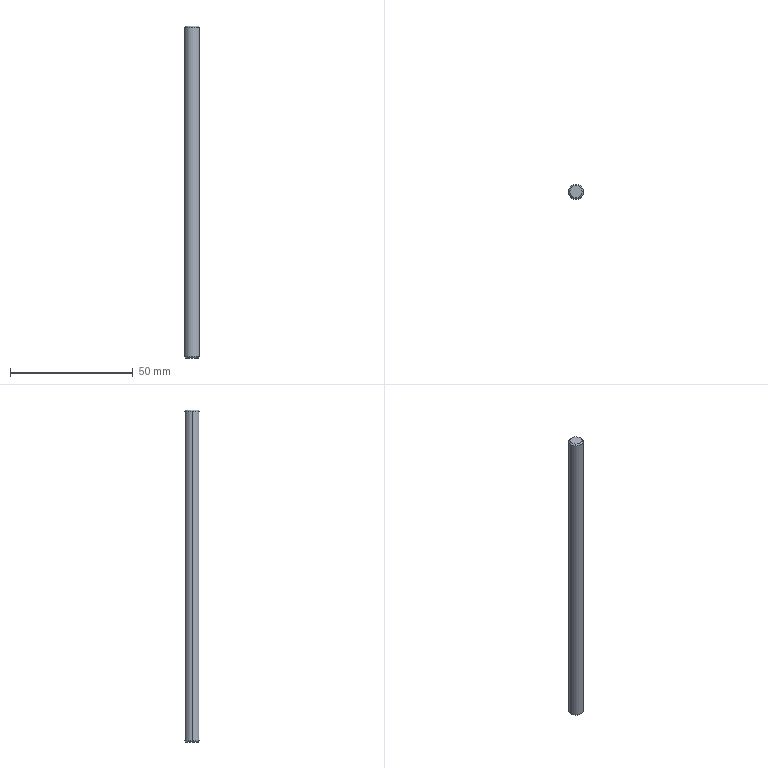Part | 1 solid | 8 faces | box 6 x 6 x 135 mm | volume 3813 mm3 | cone 4 | cylinder 2 | plane 2 | commonest cylinder face diameters 6 x2
STEP:
#1=CARTESIAN_POINT('',(2.5,0.,67.5));
#2=VERTEX_POINT('',#1);
#3=CARTESIAN_POINT('',(-2.5,0.,67.5));
#4=VERTEX_POINT('',#3);
#5=CARTESIAN_POINT('',(0.,0.,67.5));
#6=DIRECTION('',(0.,0.,1.));
#7=DIRECTION('',(1.,0.,0.));
#8=AXIS2_PLACEMENT_3D('',#5,#6,#7);
#9=CIRCLE('',#8,2.5);
#10=EDGE_CURVE('',#2,#4,#9,.T.);
#11=ORIENTED_EDGE('',*,*,#10,.F.);
#12=CARTESIAN_POINT('',(3.,0.,67.));
#13=VERTEX_POINT('',#12);
#14=CARTESIAN_POINT('',(2.5,0.,67.5));
#15=DIRECTION('',(0.7071,0.,-0.7071));
#16=VECTOR('',#15,1000.);
#17=LINE('',#14,#16);
#18=EDGE_CURVE('',#2,#13,#17,.T.);
#19=ORIENTED_EDGE('',*,*,#18,.T.);
#20=CARTESIAN_POINT('',(-3.,0.,67.));
#21=VERTEX_POINT('',#20);
#22=CARTESIAN_POINT('',(0.,0.,67.));
#23=DIRECTION('',(0.,0.,-1.));
#24=DIRECTION('',(1.,0.,0.));
#25=AXIS2_PLACEMENT_3D('',#22,#23,#24);
#26=CIRCLE('',#25,3.);
#27=EDGE_CURVE('',#21,#13,#26,.T.);
#28=ORIENTED_EDGE('',*,*,#27,.F.);
#29=CARTESIAN_POINT('',(-2.5,0.,67.5));
#30=DIRECTION('',(-0.7071,0.,-0.7071));
#31=VECTOR('',#30,1000.);
#32=LINE('',#29,#31);
#33=EDGE_CURVE('',#4,#21,#32,.T.);
#34=ORIENTED_EDGE('',*,*,#33,.F.);
#35=EDGE_LOOP('',(#11,#19,#28,#34));
#36=FACE_OUTER_BOUND('',#35,.T.);
#37=CARTESIAN_POINT('',(0.,0.,67.5));
#38=DIRECTION('',(0.,0.,-1.));
#39=DIRECTION('',(-1.,0.,0.));
#40=AXIS2_PLACEMENT_3D('',#37,#38,#39);
#41=CONICAL_SURFACE('',#40,2.5,0.7854);
#42=ADVANCED_FACE('',(#36),#41,.T.);
#43=CARTESIAN_POINT('',(-2.5,0.,-67.5));
#44=VERTEX_POINT('',#43);
#45=CARTESIAN_POINT('',(2.5,0.,-67.5));
#46=VERTEX_POINT('',#45);
#47=CARTESIAN_POINT('',(0.,0.,-67.5));
#48=DIRECTION('',(0.,0.,-1.));
#49=DIRECTION('',(1.,0.,0.));
#50=AXIS2_PLACEMENT_3D('',#47,#48,#49);
#51=CIRCLE('',#50,2.5);
#52=EDGE_CURVE('',#44,#46,#51,.T.);
#53=ORIENTED_EDGE('',*,*,#52,.F.);
#54=CARTESIAN_POINT('',(-3.,0.,-67.));
#55=VERTEX_POINT('',#54);
#56=CARTESIAN_POINT('',(-3.,0.,-67.));
#57=DIRECTION('',(-0.7071,0.,0.7071));
#58=VECTOR('',#57,1000.);
#59=LINE('',#56,#58);
#60=EDGE_CURVE('',#44,#55,#59,.T.);
#61=ORIENTED_EDGE('',*,*,#60,.T.);
#62=CARTESIAN_POINT('',(3.,0.,-67.));
#63=VERTEX_POINT('',#62);
#64=CARTESIAN_POINT('',(0.,0.,-67.));
#65=DIRECTION('',(0.,0.,1.));
#66=DIRECTION('',(1.,0.,0.));
#67=AXIS2_PLACEMENT_3D('',#64,#65,#66);
#68=CIRCLE('',#67,3.);
#69=EDGE_CURVE('',#63,#55,#68,.T.);
#70=ORIENTED_EDGE('',*,*,#69,.F.);
#71=CARTESIAN_POINT('',(3.,0.,-67.));
#72=DIRECTION('',(0.7071,0.,0.7071));
#73=VECTOR('',#72,1000.);
#74=LINE('',#71,#73);
#75=EDGE_CURVE('',#46,#63,#74,.T.);
#76=ORIENTED_EDGE('',*,*,#75,.F.);
#77=EDGE_LOOP('',(#53,#61,#70,#76));
#78=FACE_OUTER_BOUND('',#77,.T.);
#79=CARTESIAN_POINT('',(0.,0.,-67.));
#80=DIRECTION('',(0.,0.,1.));
#81=DIRECTION('',(1.,0.,0.));
#82=AXIS2_PLACEMENT_3D('',#79,#80,#81);
#83=CONICAL_SURFACE('',#82,3.,0.7854);
#84=ADVANCED_FACE('',(#78),#83,.T.);
#85=ORIENTED_EDGE('',*,*,#27,.T.);
#86=CARTESIAN_POINT('',(3.,0.,67.5));
#87=DIRECTION('',(0.,0.,-1.));
#88=VECTOR('',#87,1000.);
#89=LINE('',#86,#88);
#90=EDGE_CURVE('',#13,#63,#89,.T.);
#91=ORIENTED_EDGE('',*,*,#90,.T.);
#92=ORIENTED_EDGE('',*,*,#69,.T.);
#93=CARTESIAN_POINT('',(-3.,0.,67.5));
#94=DIRECTION('',(0.,0.,-1.));
#95=VECTOR('',#94,1000.);
#96=LINE('',#93,#95);
#97=EDGE_CURVE('',#21,#55,#96,.T.);
#98=ORIENTED_EDGE('',*,*,#97,.F.);
#99=EDGE_LOOP('',(#85,#91,#92,#98));
#100=FACE_OUTER_BOUND('',#99,.T.);
#101=CARTESIAN_POINT('',(0.,0.,67.5));
#102=DIRECTION('',(0.,0.,-1.));
#103=DIRECTION('',(-1.,0.,0.));
#104=AXIS2_PLACEMENT_3D('',#101,#102,#103);
#105=CYLINDRICAL_SURFACE('',#104,3.);
#106=ADVANCED_FACE('',(#100),#105,.T.);
#107=ORIENTED_EDGE('',*,*,#90,.F.);
#108=CARTESIAN_POINT('',(0.,0.,67.));
#109=DIRECTION('',(0.,0.,-1.));
#110=DIRECTION('',(1.,0.,0.));
#111=AXIS2_PLACEMENT_3D('',#108,#109,#110);
#112=CIRCLE('',#111,3.);
#113=EDGE_CURVE('',#13,#21,#112,.T.);
#114=ORIENTED_EDGE('',*,*,#113,.T.);
#115=ORIENTED_EDGE('',*,*,#97,.T.);
#116=CARTESIAN_POINT('',(0.,0.,-67.));
#117=DIRECTION('',(0.,0.,1.));
#118=DIRECTION('',(1.,0.,0.));
#119=AXIS2_PLACEMENT_3D('',#116,#117,#118);
#120=CIRCLE('',#119,3.);
#121=EDGE_CURVE('',#55,#63,#120,.T.);
#122=ORIENTED_EDGE('',*,*,#121,.T.);
#123=EDGE_LOOP('',(#107,#114,#115,#122));
#124=FACE_OUTER_BOUND('',#123,.T.);
#125=CARTESIAN_POINT('',(0.,0.,67.5));
#126=DIRECTION('',(0.,0.,-1.));
#127=DIRECTION('',(-1.,0.,0.));
#128=AXIS2_PLACEMENT_3D('',#125,#126,#127);
#129=CYLINDRICAL_SURFACE('',#128,3.);
#130=ADVANCED_FACE('',(#124),#129,.T.);
#131=CARTESIAN_POINT('',(0.,0.,67.5));
#132=DIRECTION('',(0.,0.,1.));
#133=DIRECTION('',(1.,0.,0.));
#134=AXIS2_PLACEMENT_3D('',#131,#132,#133);
#135=CIRCLE('',#134,2.5);
#136=EDGE_CURVE('',#4,#2,#135,.T.);
#137=ORIENTED_EDGE('',*,*,#136,.T.);
#138=ORIENTED_EDGE('',*,*,#10,.T.);
#139=EDGE_LOOP('',(#137,#138));
#140=FACE_OUTER_BOUND('',#139,.T.);
#141=CARTESIAN_POINT('',(0.,0.,67.5));
#142=DIRECTION('',(0.,0.,1.));
#143=DIRECTION('',(1.,0.,0.));
#144=AXIS2_PLACEMENT_3D('',#141,#142,#143);
#145=PLANE('',#144);
#146=ADVANCED_FACE('',(#140),#145,.T.);
#147=CARTESIAN_POINT('',(0.,0.,-67.5));
#148=DIRECTION('',(0.,0.,-1.));
#149=DIRECTION('',(1.,0.,0.));
#150=AXIS2_PLACEMENT_3D('',#147,#148,#149);
#151=CIRCLE('',#150,2.5);
#152=EDGE_CURVE('',#46,#44,#151,.T.);
#153=ORIENTED_EDGE('',*,*,#152,.T.);
#154=ORIENTED_EDGE('',*,*,#52,.T.);
#155=EDGE_LOOP('',(#153,#154));
#156=FACE_OUTER_BOUND('',#155,.T.);
#157=CARTESIAN_POINT('',(0.,0.,-67.5));
#158=DIRECTION('',(0.,0.,1.));
#159=DIRECTION('',(1.,0.,0.));
#160=AXIS2_PLACEMENT_3D('',#157,#158,#159);
#161=PLANE('',#160);
#162=ADVANCED_FACE('',(#156),#161,.F.);
#163=ORIENTED_EDGE('',*,*,#60,.F.);
#164=ORIENTED_EDGE('',*,*,#152,.F.);
#165=ORIENTED_EDGE('',*,*,#75,.T.);
#166=ORIENTED_EDGE('',*,*,#121,.F.);
#167=EDGE_LOOP('',(#163,#164,#165,#166));
#168=FACE_OUTER_BOUND('',#167,.T.);
#169=CARTESIAN_POINT('',(0.,0.,-67.));
#170=DIRECTION('',(0.,0.,1.));
#171=DIRECTION('',(1.,0.,0.));
#172=AXIS2_PLACEMENT_3D('',#169,#170,#171);
#173=CONICAL_SURFACE('',#172,3.,0.7854);
#174=ADVANCED_FACE('',(#168),#173,.T.);
#175=ORIENTED_EDGE('',*,*,#18,.F.);
#176=ORIENTED_EDGE('',*,*,#136,.F.);
#177=ORIENTED_EDGE('',*,*,#33,.T.);
#178=ORIENTED_EDGE('',*,*,#113,.F.);
#179=EDGE_LOOP('',(#175,#176,#177,#178));
#180=FACE_OUTER_BOUND('',#179,.T.);
#181=CARTESIAN_POINT('',(0.,0.,67.5));
#182=DIRECTION('',(0.,0.,-1.));
#183=DIRECTION('',(-1.,0.,0.));
#184=AXIS2_PLACEMENT_3D('',#181,#182,#183);
#185=CONICAL_SURFACE('',#184,2.5,0.7854);
#186=ADVANCED_FACE('',(#180),#185,.T.);
#187=CLOSED_SHELL('',(#42,#84,#106,#130,#146,#162,#174,#186));
#188=MANIFOLD_SOLID_BREP('',#187);
#189=CARTESIAN_POINT('',(0.,0.,0.));
#190=DIRECTION('',(0.,0.,1.));
#191=DIRECTION('',(1.,0.,0.));
#192=AXIS2_PLACEMENT_3D('',#189,#190,#191);
#193=(LENGTH_UNIT()NAMED_UNIT(*)SI_UNIT(.MILLI.,.METRE.));
#194=UNCERTAINTY_MEASURE_WITH_UNIT(LENGTH_MEASURE(0.00001),#193,'','');
#195=(NAMED_UNIT(*)PLANE_ANGLE_UNIT()SI_UNIT($,.RADIAN.));
#196=(NAMED_UNIT(*)SI_UNIT($,.STERADIAN.)SOLID_ANGLE_UNIT());
#197=(GEOMETRIC_REPRESENTATION_CONTEXT(3)GLOBAL_UNCERTAINTY_ASSIGNED_CONTEXT((#194))GLOBAL_UNIT_ASSIGNED_CONTEXT((#193,#195,#196))REPRESENTATION_CONTEXT('',''));
#198=ADVANCED_BREP_SHAPE_REPRESENTATION('',(#188,#192),#197);